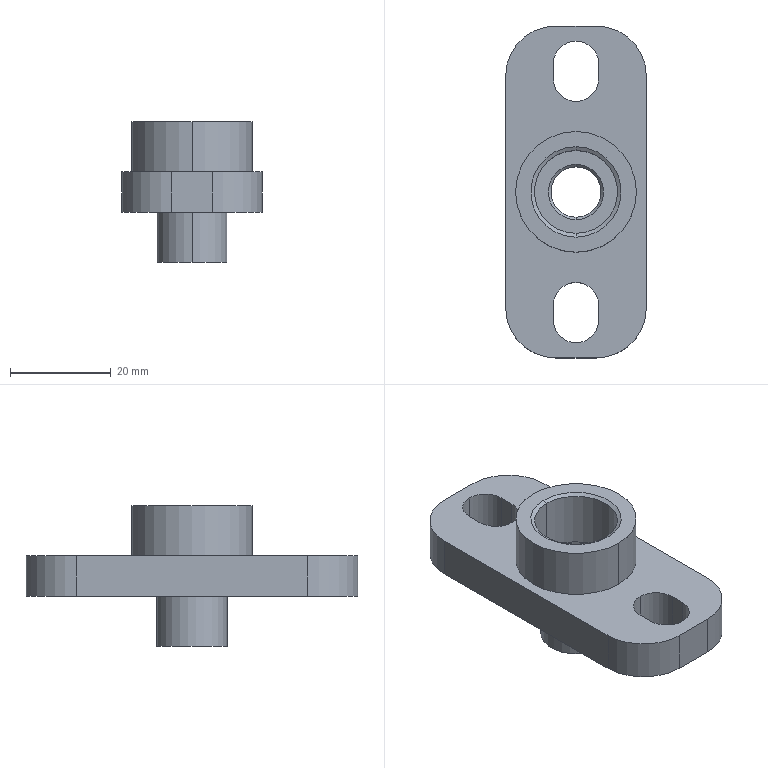Part | SolidWorks | features BaseBody 1 | 1 solid | 38 faces | box 28 x 66 x 28 mm | volume 14182 mm3 | cylinder 20 | plane 14 | cone 4 | commonest cylinder face diameters 9 x6 20 x4 10 x2 14 x2 16.5 x2 18.5 x2
STEP:
#1=CARTESIAN_POINT('',(172.5,-18.,46.8));
#2=VERTEX_POINT('',#1);
#3=CARTESIAN_POINT('',(168.,-22.5,46.8));
#4=VERTEX_POINT('',#3);
#5=CARTESIAN_POINT('',(172.5,-22.5,46.8));
#6=DIRECTION('',(0.,0.,1.));
#7=DIRECTION('',(0.,1.,0.));
#8=AXIS2_PLACEMENT_3D('',#5,#6,#7);
#9=CIRCLE('',#8,4.5);
#10=EDGE_CURVE('',#2,#4,#9,.T.);
#11=ORIENTED_EDGE('',*,*,#10,.F.);
#12=CARTESIAN_POINT('',(172.5,-18.,54.8));
#13=VERTEX_POINT('',#12);
#14=CARTESIAN_POINT('',(172.5,-18.,36.8));
#15=DIRECTION('',(0.,0.,1.));
#16=VECTOR('',#15,1000.);
#17=LINE('',#14,#16);
#18=EDGE_CURVE('',#2,#13,#17,.T.);
#19=ORIENTED_EDGE('',*,*,#18,.T.);
#20=CARTESIAN_POINT('',(168.,-22.5,54.8));
#21=VERTEX_POINT('',#20);
#22=CARTESIAN_POINT('',(172.5,-22.5,54.8));
#23=DIRECTION('',(0.,0.,1.));
#24=DIRECTION('',(0.,1.,0.));
#25=AXIS2_PLACEMENT_3D('',#22,#23,#24);
#26=CIRCLE('',#25,4.5);
#27=EDGE_CURVE('',#13,#21,#26,.T.);
#28=ORIENTED_EDGE('',*,*,#27,.T.);
#29=CARTESIAN_POINT('',(168.,-22.5,36.8));
#30=DIRECTION('',(0.,0.,1.));
#31=VECTOR('',#30,1000.);
#32=LINE('',#29,#31);
#33=EDGE_CURVE('',#4,#21,#32,.T.);
#34=ORIENTED_EDGE('',*,*,#33,.F.);
#35=EDGE_LOOP('',(#11,#19,#28,#34));
#36=FACE_OUTER_BOUND('',#35,.T.);
#37=CARTESIAN_POINT('',(172.5,-22.5,36.8));
#38=DIRECTION('',(0.,0.,1.));
#39=DIRECTION('',(0.,1.,0.));
#40=AXIS2_PLACEMENT_3D('',#37,#38,#39);
#41=CYLINDRICAL_SURFACE('',#40,4.5);
#42=ADVANCED_FACE('',(#36),#41,.F.);
#43=CARTESIAN_POINT('',(172.5,30.,46.8));
#44=VERTEX_POINT('',#43);
#45=CARTESIAN_POINT('',(168.,25.5,46.8));
#46=VERTEX_POINT('',#45);
#47=CARTESIAN_POINT('',(172.5,25.5,46.8));
#48=DIRECTION('',(0.,0.,1.));
#49=DIRECTION('',(0.,1.,0.));
#50=AXIS2_PLACEMENT_3D('',#47,#48,#49);
#51=CIRCLE('',#50,4.5);
#52=EDGE_CURVE('',#44,#46,#51,.T.);
#53=ORIENTED_EDGE('',*,*,#52,.F.);
#54=CARTESIAN_POINT('',(172.5,30.,54.8));
#55=VERTEX_POINT('',#54);
#56=CARTESIAN_POINT('',(172.5,30.,36.8));
#57=DIRECTION('',(0.,0.,1.));
#58=VECTOR('',#57,1000.);
#59=LINE('',#56,#58);
#60=EDGE_CURVE('',#44,#55,#59,.T.);
#61=ORIENTED_EDGE('',*,*,#60,.T.);
#62=CARTESIAN_POINT('',(168.,25.5,54.8));
#63=VERTEX_POINT('',#62);
#64=CARTESIAN_POINT('',(172.5,25.5,54.8));
#65=DIRECTION('',(0.,0.,1.));
#66=DIRECTION('',(0.,-1.,0.));
#67=AXIS2_PLACEMENT_3D('',#64,#65,#66);
#68=CIRCLE('',#67,4.5);
#69=EDGE_CURVE('',#55,#63,#68,.T.);
#70=ORIENTED_EDGE('',*,*,#69,.T.);
#71=CARTESIAN_POINT('',(168.,25.5,36.8));
#72=DIRECTION('',(0.,0.,1.));
#73=VECTOR('',#72,1000.);
#74=LINE('',#71,#73);
#75=EDGE_CURVE('',#46,#63,#74,.T.);
#76=ORIENTED_EDGE('',*,*,#75,.F.);
#77=EDGE_LOOP('',(#53,#61,#70,#76));
#78=FACE_OUTER_BOUND('',#77,.T.);
#79=CARTESIAN_POINT('',(172.5,25.5,36.8));
#80=DIRECTION('',(0.,0.,1.));
#81=DIRECTION('',(0.,1.,0.));
#82=AXIS2_PLACEMENT_3D('',#79,#80,#81);
#83=CYLINDRICAL_SURFACE('',#82,4.5);
#84=ADVANCED_FACE('',(#78),#83,.F.);
#85=CARTESIAN_POINT('',(172.5,-9.25,49.3));
#86=VERTEX_POINT('',#85);
#87=CARTESIAN_POINT('',(172.5,9.25,49.3));
#88=VERTEX_POINT('',#87);
#89=CARTESIAN_POINT('',(172.5,0.,49.3));
#90=DIRECTION('',(0.,0.,1.));
#91=DIRECTION('',(0.,1.,0.));
#92=AXIS2_PLACEMENT_3D('',#89,#90,#91);
#93=CIRCLE('',#92,9.25);
#94=EDGE_CURVE('',#86,#88,#93,.T.);
#95=ORIENTED_EDGE('',*,*,#94,.F.);
#96=CARTESIAN_POINT('',(172.5,-9.25,53.3));
#97=VERTEX_POINT('',#96);
#98=CARTESIAN_POINT('',(172.5,-9.25,65.548));
#99=DIRECTION('',(0.,0.,1.));
#100=VECTOR('',#99,1000.);
#101=LINE('',#98,#100);
#102=EDGE_CURVE('',#86,#97,#101,.T.);
#103=ORIENTED_EDGE('',*,*,#102,.T.);
#104=CARTESIAN_POINT('',(172.5,9.25,53.3));
#105=VERTEX_POINT('',#104);
#106=CARTESIAN_POINT('',(172.5,0.,53.3));
#107=DIRECTION('',(0.,0.,1.));
#108=DIRECTION('',(0.,1.,0.));
#109=AXIS2_PLACEMENT_3D('',#106,#107,#108);
#110=CIRCLE('',#109,9.25);
#111=EDGE_CURVE('',#97,#105,#110,.T.);
#112=ORIENTED_EDGE('',*,*,#111,.T.);
#113=CARTESIAN_POINT('',(172.5,9.25,65.548));
#114=DIRECTION('',(0.,0.,1.));
#115=VECTOR('',#114,1000.);
#116=LINE('',#113,#115);
#117=EDGE_CURVE('',#88,#105,#116,.T.);
#118=ORIENTED_EDGE('',*,*,#117,.F.);
#119=EDGE_LOOP('',(#95,#103,#112,#118));
#120=FACE_OUTER_BOUND('',#119,.T.);
#121=CARTESIAN_POINT('',(172.5,0.,65.548));
#122=DIRECTION('',(0.,0.,1.));
#123=DIRECTION('',(0.,1.,0.));
#124=AXIS2_PLACEMENT_3D('',#121,#122,#123);
#125=CYLINDRICAL_SURFACE('',#124,9.25);
#126=ADVANCED_FACE('',(#120),#125,.F.);
#127=CARTESIAN_POINT('',(172.5,-5.,48.8));
#128=VERTEX_POINT('',#127);
#129=CARTESIAN_POINT('',(172.5,5.,48.8));
#130=VERTEX_POINT('',#129);
#131=CARTESIAN_POINT('',(172.5,0.,48.8));
#132=DIRECTION('',(0.,0.,1.));
#133=DIRECTION('',(0.,-1.,0.));
#134=AXIS2_PLACEMENT_3D('',#131,#132,#133);
#135=CIRCLE('',#134,5.);
#136=EDGE_CURVE('',#128,#130,#135,.T.);
#137=ORIENTED_EDGE('',*,*,#136,.F.);
#138=CARTESIAN_POINT('',(172.5,-5.5,49.3));
#139=VERTEX_POINT('',#138);
#140=CARTESIAN_POINT('',(172.5,-5.,48.8));
#141=DIRECTION('',(0.,-0.7071,0.7071));
#142=VECTOR('',#141,1000.);
#143=LINE('',#140,#142);
#144=EDGE_CURVE('',#128,#139,#143,.T.);
#145=ORIENTED_EDGE('',*,*,#144,.T.);
#146=CARTESIAN_POINT('',(172.5,5.5,49.3));
#147=VERTEX_POINT('',#146);
#148=CARTESIAN_POINT('',(172.5,0.,49.3));
#149=DIRECTION('',(0.,0.,-1.));
#150=DIRECTION('',(0.,-1.,0.));
#151=AXIS2_PLACEMENT_3D('',#148,#149,#150);
#152=CIRCLE('',#151,5.5);
#153=EDGE_CURVE('',#147,#139,#152,.T.);
#154=ORIENTED_EDGE('',*,*,#153,.F.);
#155=CARTESIAN_POINT('',(172.5,5.,48.8));
#156=DIRECTION('',(0.,0.7071,0.7071));
#157=VECTOR('',#156,1000.);
#158=LINE('',#155,#157);
#159=EDGE_CURVE('',#130,#147,#158,.T.);
#160=ORIENTED_EDGE('',*,*,#159,.F.);
#161=EDGE_LOOP('',(#137,#145,#154,#160));
#162=FACE_OUTER_BOUND('',#161,.T.);
#163=CARTESIAN_POINT('',(172.5,0.,48.8));
#164=DIRECTION('',(0.,0.,1.));
#165=DIRECTION('',(0.,1.,0.));
#166=AXIS2_PLACEMENT_3D('',#163,#164,#165);
#167=CONICAL_SURFACE('',#166,5.,0.7854);
#168=ADVANCED_FACE('',(#162),#167,.F.);
#169=CARTESIAN_POINT('',(172.5,-8.25,64.367));
#170=VERTEX_POINT('',#169);
#171=CARTESIAN_POINT('',(172.5,8.25,64.367));
#172=VERTEX_POINT('',#171);
#173=CARTESIAN_POINT('',(172.5,0.,64.367));
#174=DIRECTION('',(0.,0.,1.));
#175=DIRECTION('',(0.,1.,0.));
#176=AXIS2_PLACEMENT_3D('',#173,#174,#175);
#177=CIRCLE('',#176,8.25);
#178=EDGE_CURVE('',#170,#172,#177,.T.);
#179=ORIENTED_EDGE('',*,*,#178,.F.);
#180=CARTESIAN_POINT('',(172.5,-9.,64.8));
#181=VERTEX_POINT('',#180);
#182=CARTESIAN_POINT('',(172.5,-9.,64.8));
#183=DIRECTION('',(0.,-0.866,0.5));
#184=VECTOR('',#183,1000.);
#185=LINE('',#182,#184);
#186=EDGE_CURVE('',#170,#181,#185,.T.);
#187=ORIENTED_EDGE('',*,*,#186,.T.);
#188=CARTESIAN_POINT('',(172.5,9.,64.8));
#189=VERTEX_POINT('',#188);
#190=CARTESIAN_POINT('',(172.5,0.,64.8));
#191=DIRECTION('',(0.,0.,1.));
#192=DIRECTION('',(0.,1.,0.));
#193=AXIS2_PLACEMENT_3D('',#190,#191,#192);
#194=CIRCLE('',#193,9.);
#195=EDGE_CURVE('',#181,#189,#194,.T.);
#196=ORIENTED_EDGE('',*,*,#195,.T.);
#197=CARTESIAN_POINT('',(172.5,9.,64.8));
#198=DIRECTION('',(0.,0.866,0.5));
#199=VECTOR('',#198,1000.);
#200=LINE('',#197,#199);
#201=EDGE_CURVE('',#172,#189,#200,.T.);
#202=ORIENTED_EDGE('',*,*,#201,.F.);
#203=EDGE_LOOP('',(#179,#187,#196,#202));
#204=FACE_OUTER_BOUND('',#203,.T.);
#205=CARTESIAN_POINT('',(172.5,0.,64.8));
#206=DIRECTION('',(0.,0.,1.));
#207=DIRECTION('',(0.,1.,0.));
#208=AXIS2_PLACEMENT_3D('',#205,#206,#207);
#209=CONICAL_SURFACE('',#208,9.,1.047);
#210=ADVANCED_FACE('',(#204),#209,.F.);
#211=CARTESIAN_POINT('',(172.5,-5.,36.8));
#212=VERTEX_POINT('',#211);
#213=CARTESIAN_POINT('',(172.5,5.,36.8));
#214=VERTEX_POINT('',#213);
#215=CARTESIAN_POINT('',(172.5,0.,36.8));
#216=DIRECTION('',(0.,0.,1.));
#217=DIRECTION('',(0.,1.,0.));
#218=AXIS2_PLACEMENT_3D('',#215,#216,#217);
#219=CIRCLE('',#218,5.);
#220=EDGE_CURVE('',#212,#214,#219,.T.);
#221=ORIENTED_EDGE('',*,*,#220,.F.);
#222=CARTESIAN_POINT('',(172.5,-5.,36.8));
#223=DIRECTION('',(0.,0.,1.));
#224=VECTOR('',#223,1000.);
#225=LINE('',#222,#224);
#226=EDGE_CURVE('',#212,#128,#225,.T.);
#227=ORIENTED_EDGE('',*,*,#226,.T.);
#228=ORIENTED_EDGE('',*,*,#136,.T.);
#229=CARTESIAN_POINT('',(172.5,5.,36.8));
#230=DIRECTION('',(0.,0.,1.));
#231=VECTOR('',#230,1000.);
#232=LINE('',#229,#231);
#233=EDGE_CURVE('',#214,#130,#232,.T.);
#234=ORIENTED_EDGE('',*,*,#233,.F.);
#235=EDGE_LOOP('',(#221,#227,#228,#234));
#236=FACE_OUTER_BOUND('',#235,.T.);
#237=CARTESIAN_POINT('',(172.5,0.,36.8));
#238=DIRECTION('',(0.,0.,1.));
#239=DIRECTION('',(0.,1.,0.));
#240=AXIS2_PLACEMENT_3D('',#237,#238,#239);
#241=CYLINDRICAL_SURFACE('',#240,5.);
#242=ADVANCED_FACE('',(#236),#241,.F.);
#243=CARTESIAN_POINT('',(172.5,7.,36.8));
#244=VERTEX_POINT('',#243);
#245=CARTESIAN_POINT('',(172.5,-7.,36.8));
#246=VERTEX_POINT('',#245);
#247=CARTESIAN_POINT('',(172.5,0.,36.8));
#248=DIRECTION('',(0.,0.,1.));
#249=DIRECTION('',(0.,1.,0.));
#250=AXIS2_PLACEMENT_3D('',#247,#248,#249);
#251=CIRCLE('',#250,7.);
#252=EDGE_CURVE('',#244,#246,#251,.T.);
#253=ORIENTED_EDGE('',*,*,#252,.T.);
#254=CARTESIAN_POINT('',(172.5,-7.,46.8));
#255=VERTEX_POINT('',#254);
#256=CARTESIAN_POINT('',(172.5,-7.,-10.999));
#257=DIRECTION('',(0.,0.,1.));
#258=VECTOR('',#257,1000.);
#259=LINE('',#256,#258);
#260=EDGE_CURVE('',#246,#255,#259,.T.);
#261=ORIENTED_EDGE('',*,*,#260,.T.);
#262=CARTESIAN_POINT('',(172.5,7.,46.8));
#263=VERTEX_POINT('',#262);
#264=CARTESIAN_POINT('',(172.5,0.,46.8));
#265=DIRECTION('',(0.,0.,-1.));
#266=DIRECTION('',(0.,1.,0.));
#267=AXIS2_PLACEMENT_3D('',#264,#265,#266);
#268=CIRCLE('',#267,7.);
#269=EDGE_CURVE('',#255,#263,#268,.T.);
#270=ORIENTED_EDGE('',*,*,#269,.T.);
#271=CARTESIAN_POINT('',(172.5,7.,-10.999));
#272=DIRECTION('',(0.,0.,1.));
#273=VECTOR('',#272,1000.);
#274=LINE('',#271,#273);
#275=EDGE_CURVE('',#244,#263,#274,.T.);
#276=ORIENTED_EDGE('',*,*,#275,.F.);
#277=EDGE_LOOP('',(#253,#261,#270,#276));
#278=FACE_OUTER_BOUND('',#277,.T.);
#279=CARTESIAN_POINT('',(172.5,0.,-10.999));
#280=DIRECTION('',(0.,0.,1.));
#281=DIRECTION('',(0.,1.,0.));
#282=AXIS2_PLACEMENT_3D('',#279,#280,#281);
#283=CYLINDRICAL_SURFACE('',#282,7.);
#284=ADVANCED_FACE('',(#278),#283,.T.);
#285=CARTESIAN_POINT('',(172.5,12.,64.8));
#286=VERTEX_POINT('',#285);
#287=CARTESIAN_POINT('',(172.5,-12.,64.8));
#288=VERTEX_POINT('',#287);
#289=CARTESIAN_POINT('',(172.5,0.,64.8));
#290=DIRECTION('',(0.,0.,1.));
#291=DIRECTION('',(0.,1.,0.));
#292=AXIS2_PLACEMENT_3D('',#289,#290,#291);
#293=CIRCLE('',#292,12.);
#294=EDGE_CURVE('',#286,#288,#293,.T.);
#295=ORIENTED_EDGE('',*,*,#294,.F.);
#296=CARTESIAN_POINT('',(172.5,12.,54.8));
#297=VERTEX_POINT('',#296);
#298=CARTESIAN_POINT('',(172.5,12.,64.8));
#299=DIRECTION('',(0.,0.,-1.));
#300=VECTOR('',#299,1000.);
#301=LINE('',#298,#300);
#302=EDGE_CURVE('',#286,#297,#301,.T.);
#303=ORIENTED_EDGE('',*,*,#302,.T.);
#304=CARTESIAN_POINT('',(172.5,-12.,54.8));
#305=VERTEX_POINT('',#304);
#306=CARTESIAN_POINT('',(172.5,0.,54.8));
#307=DIRECTION('',(0.,0.,1.));
#308=DIRECTION('',(0.,1.,0.));
#309=AXIS2_PLACEMENT_3D('',#306,#307,#308);
#310=CIRCLE('',#309,12.);
#311=EDGE_CURVE('',#297,#305,#310,.T.);
#312=ORIENTED_EDGE('',*,*,#311,.T.);
#313=CARTESIAN_POINT('',(172.5,-12.,64.8));
#314=DIRECTION('',(0.,0.,-1.));
#315=VECTOR('',#314,1000.);
#316=LINE('',#313,#315);
#317=EDGE_CURVE('',#288,#305,#316,.T.);
#318=ORIENTED_EDGE('',*,*,#317,.F.);
#319=EDGE_LOOP('',(#295,#303,#312,#318));
#320=FACE_OUTER_BOUND('',#319,.T.);
#321=CARTESIAN_POINT('',(172.5,0.,64.8));
#322=DIRECTION('',(0.,0.,-1.));
#323=DIRECTION('',(0.,-1.,0.));
#324=AXIS2_PLACEMENT_3D('',#321,#322,#323);
#325=CYLINDRICAL_SURFACE('',#324,12.);
#326=ADVANCED_FACE('',(#320),#325,.T.);
#327=CARTESIAN_POINT('',(172.5,-8.25,53.3));
#328=VERTEX_POINT('',#327);
#329=CARTESIAN_POINT('',(172.5,8.25,53.3));
#330=VERTEX_POINT('',#329);
#331=CARTESIAN_POINT('',(172.5,0.,53.3));
#332=DIRECTION('',(0.,0.,1.));
#333=DIRECTION('',(0.,-1.,0.));
#334=AXIS2_PLACEMENT_3D('',#331,#332,#333);
#335=CIRCLE('',#334,8.25);
#336=EDGE_CURVE('',#328,#330,#335,.T.);
#337=ORIENTED_EDGE('',*,*,#336,.F.);
#338=CARTESIAN_POINT('',(172.5,-8.25,64.8));
#339=DIRECTION('',(0.,0.,1.));
#340=VECTOR('',#339,1000.);
#341=LINE('',#338,#340);
#342=EDGE_CURVE('',#328,#170,#341,.T.);
#343=ORIENTED_EDGE('',*,*,#342,.T.);
#344=ORIENTED_EDGE('',*,*,#178,.T.);
#345=CARTESIAN_POINT('',(172.5,8.25,64.8));
#346=DIRECTION('',(0.,0.,1.));
#347=VECTOR('',#346,1000.);
#348=LINE('',#345,#347);
#349=EDGE_CURVE('',#330,#172,#348,.T.);
#350=ORIENTED_EDGE('',*,*,#349,.F.);
#351=EDGE_LOOP('',(#337,#343,#344,#350));
#352=FACE_OUTER_BOUND('',#351,.T.);
#353=CARTESIAN_POINT('',(172.5,0.,64.8));
#354=DIRECTION('',(0.,0.,1.));
#355=DIRECTION('',(0.,1.,0.));
#356=AXIS2_PLACEMENT_3D('',#353,#354,#355);
#357=CYLINDRICAL_SURFACE('',#356,8.25);
#358=ADVANCED_FACE('',(#352),#357,.F.);
#359=ORIENTED_EDGE('',*,*,#342,.F.);
#360=CARTESIAN_POINT('',(172.5,0.,53.3));
#361=DIRECTION('',(0.,0.,1.));
#362=DIRECTION('',(0.,-1.,0.));
#363=AXIS2_PLACEMENT_3D('',#360,#361,#362);
#364=CIRCLE('',#363,8.25);
#365=EDGE_CURVE('',#330,#328,#364,.T.);
#366=ORIENTED_EDGE('',*,*,#365,.F.);
#367=ORIENTED_EDGE('',*,*,#349,.T.);
#368=CARTESIAN_POINT('',(172.5,0.,64.367));
#369=DIRECTION('',(0.,0.,1.));
#370=DIRECTION('',(0.,1.,0.));
#371=AXIS2_PLACEMENT_3D('',#368,#369,#370);
#372=CIRCLE('',#371,8.25);
#373=EDGE_CURVE('',#172,#170,#372,.T.);
#374=ORIENTED_EDGE('',*,*,#373,.T.);
#375=EDGE_LOOP('',(#359,#366,#367,#374));
#376=FACE_OUTER_BOUND('',#375,.T.);
#377=CARTESIAN_POINT('',(172.5,0.,64.8));
#378=DIRECTION('',(0.,0.,1.));
#379=DIRECTION('',(0.,1.,0.));
#380=AXIS2_PLACEMENT_3D('',#377,#378,#379);
#381=CYLINDRICAL_SURFACE('',#380,8.25);
#382=ADVANCED_FACE('',(#376),#381,.F.);
#383=CARTESIAN_POINT('',(168.,-25.5,46.8));
#384=VERTEX_POINT('',#383);
#385=CARTESIAN_POINT('',(168.,23.,46.8));
#386=DIRECTION('',(0.,-1.,0.));
#387=VECTOR('',#386,1000.);
#388=LINE('',#385,#387);
#389=EDGE_CURVE('',#4,#384,#388,.T.);
#390=ORIENTED_EDGE('',*,*,#389,.T.);
#391=CARTESIAN_POINT('',(177.,-25.5,46.8));
#392=VERTEX_POINT('',#391);
#393=CARTESIAN_POINT('',(172.5,-25.5,46.8));
#394=DIRECTION('',(0.,0.,1.));
#395=DIRECTION('',(0.,1.,0.));
#396=AXIS2_PLACEMENT_3D('',#393,#394,#395);
#397=CIRCLE('',#396,4.5);
#398=EDGE_CURVE('',#384,#392,#397,.T.);
#399=ORIENTED_EDGE('',*,*,#398,.T.);
#400=CARTESIAN_POINT('',(177.,-22.5,46.8));
#401=VERTEX_POINT('',#400);
#402=CARTESIAN_POINT('',(177.,23.,46.8));
#403=DIRECTION('',(0.,1.,0.));
#404=VECTOR('',#403,1000.);
#405=LINE('',#402,#404);
#406=EDGE_CURVE('',#392,#401,#405,.T.);
#407=ORIENTED_EDGE('',*,*,#406,.T.);
#408=CARTESIAN_POINT('',(172.5,-22.5,46.8));
#409=DIRECTION('',(0.,0.,1.));
#410=DIRECTION('',(0.,1.,0.));
#411=AXIS2_PLACEMENT_3D('',#408,#409,#410);
#412=CIRCLE('',#411,4.5);
#413=EDGE_CURVE('',#401,#2,#412,.T.);
#414=ORIENTED_EDGE('',*,*,#413,.T.);
#415=ORIENTED_EDGE('',*,*,#10,.T.);
#416=EDGE_LOOP('',(#390,#399,#407,#414,#415));
#417=FACE_BOUND('',#416,.T.);
#418=CARTESIAN_POINT('',(168.,22.5,46.8));
#419=VERTEX_POINT('',#418);
#420=CARTESIAN_POINT('',(168.,23.,46.8));
#421=DIRECTION('',(0.,-1.,0.));
#422=VECTOR('',#421,1000.);
#423=LINE('',#420,#422);
#424=EDGE_CURVE('',#46,#419,#423,.T.);
#425=ORIENTED_EDGE('',*,*,#424,.T.);
#426=CARTESIAN_POINT('',(177.,22.5,46.8));
#427=VERTEX_POINT('',#426);
#428=CARTESIAN_POINT('',(172.5,22.5,46.8));
#429=DIRECTION('',(0.,0.,1.));
#430=DIRECTION('',(0.,1.,0.));
#431=AXIS2_PLACEMENT_3D('',#428,#429,#430);
#432=CIRCLE('',#431,4.5);
#433=EDGE_CURVE('',#419,#427,#432,.T.);
#434=ORIENTED_EDGE('',*,*,#433,.T.);
#435=CARTESIAN_POINT('',(177.,25.5,46.8));
#436=VERTEX_POINT('',#435);
#437=CARTESIAN_POINT('',(177.,23.,46.8));
#438=DIRECTION('',(0.,1.,0.));
#439=VECTOR('',#438,1000.);
#440=LINE('',#437,#439);
#441=EDGE_CURVE('',#427,#436,#440,.T.);
#442=ORIENTED_EDGE('',*,*,#441,.T.);
#443=CARTESIAN_POINT('',(172.5,25.5,46.8));
#444=DIRECTION('',(0.,0.,1.));
#445=DIRECTION('',(0.,1.,0.));
#446=AXIS2_PLACEMENT_3D('',#443,#444,#445);
#447=CIRCLE('',#446,4.5);
#448=EDGE_CURVE('',#436,#44,#447,.T.);
#449=ORIENTED_EDGE('',*,*,#448,.T.);
#450=ORIENTED_EDGE('',*,*,#52,.T.);
#451=EDGE_LOOP('',(#425,#434,#442,#449,#450));
#452=FACE_BOUND('',#451,.T.);
#453=CARTESIAN_POINT('',(168.5,33.,46.8));
#454=VERTEX_POINT('',#453);
#455=CARTESIAN_POINT('',(158.5,23.,46.8));
#456=VERTEX_POINT('',#455);
#457=CARTESIAN_POINT('',(168.5,23.,46.8));
#458=DIRECTION('',(0.,0.,1.));
#459=DIRECTION('',(0.,1.,0.));
#460=AXIS2_PLACEMENT_3D('',#457,#458,#459);
#461=CIRCLE('',#460,10.);
#462=EDGE_CURVE('',#454,#456,#461,.T.);
#463=ORIENTED_EDGE('',*,*,#462,.F.);
#464=CARTESIAN_POINT('',(176.5,33.,46.8));
#465=VERTEX_POINT('',#464);
#466=CARTESIAN_POINT('',(168.5,33.,46.8));
#467=DIRECTION('',(-1.,0.,0.));
#468=VECTOR('',#467,1000.);
#469=LINE('',#466,#468);
#470=EDGE_CURVE('',#465,#454,#469,.T.);
#471=ORIENTED_EDGE('',*,*,#470,.F.);
#472=CARTESIAN_POINT('',(186.5,23.,46.8));
#473=VERTEX_POINT('',#472);
#474=CARTESIAN_POINT('',(176.5,23.,46.8));
#475=DIRECTION('',(0.,0.,1.));
#476=DIRECTION('',(0.,1.,0.));
#477=AXIS2_PLACEMENT_3D('',#474,#475,#476);
#478=CIRCLE('',#477,10.);
#479=EDGE_CURVE('',#473,#465,#478,.T.);
#480=ORIENTED_EDGE('',*,*,#479,.F.);
#481=CARTESIAN_POINT('',(186.5,-23.,46.8));
#482=VERTEX_POINT('',#481);
#483=CARTESIAN_POINT('',(186.5,-23.,46.8));
#484=DIRECTION('',(0.,1.,0.));
#485=VECTOR('',#484,1000.);
#486=LINE('',#483,#485);
#487=EDGE_CURVE('',#482,#473,#486,.T.);
#488=ORIENTED_EDGE('',*,*,#487,.F.);
#489=CARTESIAN_POINT('',(176.5,-33.,46.8));
#490=VERTEX_POINT('',#489);
#491=CARTESIAN_POINT('',(176.5,-23.,46.8));
#492=DIRECTION('',(0.,0.,1.));
#493=DIRECTION('',(0.,1.,0.));
#494=AXIS2_PLACEMENT_3D('',#491,#492,#493);
#495=CIRCLE('',#494,10.);
#496=EDGE_CURVE('',#490,#482,#495,.T.);
#497=ORIENTED_EDGE('',*,*,#496,.F.);
#498=CARTESIAN_POINT('',(168.5,-33.,46.8));
#499=VERTEX_POINT('',#498);
#500=CARTESIAN_POINT('',(168.5,-33.,46.8));
#501=DIRECTION('',(1.,0.,0.));
#502=VECTOR('',#501,1000.);
#503=LINE('',#500,#502);
#504=EDGE_CURVE('',#499,#490,#503,.T.);
#505=ORIENTED_EDGE('',*,*,#504,.F.);
#506=CARTESIAN_POINT('',(158.5,-23.,46.8));
#507=VERTEX_POINT('',#506);
#508=CARTESIAN_POINT('',(168.5,-23.,46.8));
#509=DIRECTION('',(0.,0.,1.));
#510=DIRECTION('',(0.,1.,0.));
#511=AXIS2_PLACEMENT_3D('',#508,#509,#510);
#512=CIRCLE('',#511,10.);
#513=EDGE_CURVE('',#507,#499,#512,.T.);
#514=ORIENTED_EDGE('',*,*,#513,.F.);
#515=CARTESIAN_POINT('',(158.5,-23.,46.8));
#516=DIRECTION('',(0.,-1.,0.));
#517=VECTOR('',#516,1000.);
#518=LINE('',#515,#517);
#519=EDGE_CURVE('',#456,#507,#518,.T.);
#520=ORIENTED_EDGE('',*,*,#519,.F.);
#521=EDGE_LOOP('',(#463,#471,#480,#488,#497,#505,#514,#520));
#522=FACE_OUTER_BOUND('',#521,.T.);
#523=CARTESIAN_POINT('',(172.5,0.,46.8));
#524=DIRECTION('',(0.,0.,-1.));
#525=DIRECTION('',(0.,1.,0.));
#526=AXIS2_PLACEMENT_3D('',#523,#524,#525);
#527=CIRCLE('',#526,7.);
#528=EDGE_CURVE('',#263,#255,#527,.T.);
#529=ORIENTED_EDGE('',*,*,#528,.F.);
#530=ORIENTED_EDGE('',*,*,#269,.F.);
#531=EDGE_LOOP('',(#529,#530));
#532=FACE_BOUND('',#531,.T.);
#533=CARTESIAN_POINT('',(168.5,23.,46.8));
#534=DIRECTION('',(0.,0.,1.));
#535=DIRECTION('',(0.,1.,0.));
#536=AXIS2_PLACEMENT_3D('',#533,#534,#535);
#537=PLANE('',#536);
#538=ADVANCED_FACE('',(#417,#452,#522,#532),#537,.F.);
#539=CARTESIAN_POINT('',(168.,-25.5,54.8));
#540=VERTEX_POINT('',#539);
#541=CARTESIAN_POINT('',(177.,-25.5,54.8));
#542=VERTEX_POINT('',#541);
#543=CARTESIAN_POINT('',(172.5,-25.5,54.8));
#544=DIRECTION('',(0.,0.,1.));
#545=DIRECTION('',(0.,1.,0.));
#546=AXIS2_PLACEMENT_3D('',#543,#544,#545);
#547=CIRCLE('',#546,4.5);
#548=EDGE_CURVE('',#540,#542,#547,.T.);
#549=ORIENTED_EDGE('',*,*,#548,.F.);
#550=CARTESIAN_POINT('',(168.,-25.5,54.8));
#551=DIRECTION('',(0.,-1.,0.));
#552=VECTOR('',#551,1000.);
#553=LINE('',#550,#552);
#554=EDGE_CURVE('',#21,#540,#553,.T.);
#555=ORIENTED_EDGE('',*,*,#554,.F.);
#556=ORIENTED_EDGE('',*,*,#27,.F.);
#557=CARTESIAN_POINT('',(177.,-22.5,54.8));
#558=VERTEX_POINT('',#557);
#559=CARTESIAN_POINT('',(172.5,-22.5,54.8));
#560=DIRECTION('',(0.,0.,1.));
#561=DIRECTION('',(0.,1.,0.));
#562=AXIS2_PLACEMENT_3D('',#559,#560,#561);
#563=CIRCLE('',#562,4.5);
#564=EDGE_CURVE('',#558,#13,#563,.T.);
#565=ORIENTED_EDGE('',*,*,#564,.F.);
#566=CARTESIAN_POINT('',(177.,-22.5,54.8));
#567=DIRECTION('',(0.,1.,0.));
#568=VECTOR('',#567,1000.);
#569=LINE('',#566,#568);
#570=EDGE_CURVE('',#542,#558,#569,.T.);
#571=ORIENTED_EDGE('',*,*,#570,.F.);
#572=EDGE_LOOP('',(#549,#555,#556,#565,#571));
#573=FACE_BOUND('',#572,.T.);
#574=CARTESIAN_POINT('',(168.,22.5,54.8));
#575=VERTEX_POINT('',#574);
#576=CARTESIAN_POINT('',(177.,22.5,54.8));
#577=VERTEX_POINT('',#576);
#578=CARTESIAN_POINT('',(172.5,22.5,54.8));
#579=DIRECTION('',(0.,0.,1.));
#580=DIRECTION('',(0.,-1.,0.));
#581=AXIS2_PLACEMENT_3D('',#578,#579,#580);
#582=CIRCLE('',#581,4.5);
#583=EDGE_CURVE('',#575,#577,#582,.T.);
#584=ORIENTED_EDGE('',*,*,#583,.F.);
#585=CARTESIAN_POINT('',(168.,25.5,54.8));
#586=DIRECTION('',(0.,-1.,0.));
#587=VECTOR('',#586,1000.);
#588=LINE('',#585,#587);
#589=EDGE_CURVE('',#63,#575,#588,.T.);
#590=ORIENTED_EDGE('',*,*,#589,.F.);
#591=ORIENTED_EDGE('',*,*,#69,.F.);
#592=CARTESIAN_POINT('',(177.,25.5,54.8));
#593=VERTEX_POINT('',#592);
#594=CARTESIAN_POINT('',(172.5,25.5,54.8));
#595=DIRECTION('',(0.,0.,1.));
#596=DIRECTION('',(0.,-1.,0.));
#597=AXIS2_PLACEMENT_3D('',#594,#595,#596);
#598=CIRCLE('',#597,4.5);
#599=EDGE_CURVE('',#593,#55,#598,.T.);
#600=ORIENTED_EDGE('',*,*,#599,.F.);
#601=CARTESIAN_POINT('',(177.,22.5,54.8));
#602=DIRECTION('',(0.,1.,0.));
#603=VECTOR('',#602,1000.);
#604=LINE('',#601,#603);
#605=EDGE_CURVE('',#577,#593,#604,.T.);
#606=ORIENTED_EDGE('',*,*,#605,.F.);
#607=EDGE_LOOP('',(#584,#590,#591,#600,#606));
#608=FACE_BOUND('',#607,.T.);
#609=CARTESIAN_POINT('',(168.5,33.,54.8));
#610=VERTEX_POINT('',#609);
#611=CARTESIAN_POINT('',(158.5,23.,54.8));
#612=VERTEX_POINT('',#611);
#613=CARTESIAN_POINT('',(168.5,23.,54.8));
#614=DIRECTION('',(0.,0.,1.));
#615=DIRECTION('',(0.,1.,0.));
#616=AXIS2_PLACEMENT_3D('',#613,#614,#615);
#617=CIRCLE('',#616,10.);
#618=EDGE_CURVE('',#610,#612,#617,.T.);
#619=ORIENTED_EDGE('',*,*,#618,.T.);
#620=CARTESIAN_POINT('',(158.5,-23.,54.8));
#621=VERTEX_POINT('',#620);
#622=CARTESIAN_POINT('',(158.5,-23.,54.8));
#623=DIRECTION('',(0.,-1.,0.));
#624=VECTOR('',#623,1000.);
#625=LINE('',#622,#624);
#626=EDGE_CURVE('',#612,#621,#625,.T.);
#627=ORIENTED_EDGE('',*,*,#626,.T.);
#628=CARTESIAN_POINT('',(168.5,-33.,54.8));
#629=VERTEX_POINT('',#628);
#630=CARTESIAN_POINT('',(168.5,-23.,54.8));
#631=DIRECTION('',(0.,0.,1.));
#632=DIRECTION('',(0.,1.,0.));
#633=AXIS2_PLACEMENT_3D('',#630,#631,#632);
#634=CIRCLE('',#633,10.);
#635=EDGE_CURVE('',#621,#629,#634,.T.);
#636=ORIENTED_EDGE('',*,*,#635,.T.);
#637=CARTESIAN_POINT('',(176.5,-33.,54.8));
#638=VERTEX_POINT('',#637);
#639=CARTESIAN_POINT('',(168.5,-33.,54.8));
#640=DIRECTION('',(1.,0.,0.));
#641=VECTOR('',#640,1000.);
#642=LINE('',#639,#641);
#643=EDGE_CURVE('',#629,#638,#642,.T.);
#644=ORIENTED_EDGE('',*,*,#643,.T.);
#645=CARTESIAN_POINT('',(186.5,-23.,54.8));
#646=VERTEX_POINT('',#645);
#647=CARTESIAN_POINT('',(176.5,-23.,54.8));
#648=DIRECTION('',(0.,0.,1.));
#649=DIRECTION('',(0.,1.,0.));
#650=AXIS2_PLACEMENT_3D('',#647,#648,#649);
#651=CIRCLE('',#650,10.);
#652=EDGE_CURVE('',#638,#646,#651,.T.);
#653=ORIENTED_EDGE('',*,*,#652,.T.);
#654=CARTESIAN_POINT('',(186.5,23.,54.8));
#655=VERTEX_POINT('',#654);
#656=CARTESIAN_POINT('',(186.5,-23.,54.8));
#657=DIRECTION('',(0.,1.,0.));
#658=VECTOR('',#657,1000.);
#659=LINE('',#656,#658);
#660=EDGE_CURVE('',#646,#655,#659,.T.);
#661=ORIENTED_EDGE('',*,*,#660,.T.);
#662=CARTESIAN_POINT('',(176.5,33.,54.8));
#663=VERTEX_POINT('',#662);
#664=CARTESIAN_POINT('',(176.5,23.,54.8));
#665=DIRECTION('',(0.,0.,1.));
#666=DIRECTION('',(0.,1.,0.));
#667=AXIS2_PLACEMENT_3D('',#664,#665,#666);
#668=CIRCLE('',#667,10.);
#669=EDGE_CURVE('',#655,#663,#668,.T.);
#670=ORIENTED_EDGE('',*,*,#669,.T.);
#671=CARTESIAN_POINT('',(168.5,33.,54.8));
#672=DIRECTION('',(-1.,0.,0.));
#673=VECTOR('',#672,1000.);
#674=LINE('',#671,#673);
#675=EDGE_CURVE('',#663,#610,#674,.T.);
#676=ORIENTED_EDGE('',*,*,#675,.T.);
#677=EDGE_LOOP('',(#619,#627,#636,#644,#653,#661,#670,#676));
#678=FACE_OUTER_BOUND('',#677,.T.);
#679=CARTESIAN_POINT('',(172.5,0.,54.8));
#680=DIRECTION('',(0.,0.,1.));
#681=DIRECTION('',(0.,1.,0.));
#682=AXIS2_PLACEMENT_3D('',#679,#680,#681);
#683=CIRCLE('',#682,12.);
#684=EDGE_CURVE('',#305,#297,#683,.T.);
#685=ORIENTED_EDGE('',*,*,#684,.F.);
#686=ORIENTED_EDGE('',*,*,#311,.F.);
#687=EDGE_LOOP('',(#685,#686));
#688=FACE_BOUND('',#687,.T.);
#689=CARTESIAN_POINT('',(168.5,23.,54.8));
#690=DIRECTION('',(0.,0.,1.));
#691=DIRECTION('',(0.,1.,0.));
#692=AXIS2_PLACEMENT_3D('',#689,#690,#691);
#693=PLANE('',#692);
#694=ADVANCED_FACE('',(#573,#608,#678,#688),#693,.T.);
#695=ORIENTED_EDGE('',*,*,#462,.T.);
#696=CARTESIAN_POINT('',(158.5,23.,54.8));
#697=DIRECTION('',(0.,0.,-1.));
#698=VECTOR('',#697,1000.);
#699=LINE('',#696,#698);
#700=EDGE_CURVE('',#612,#456,#699,.T.);
#701=ORIENTED_EDGE('',*,*,#700,.F.);
#702=ORIENTED_EDGE('',*,*,#618,.F.);
#703=CARTESIAN_POINT('',(168.5,33.,54.8));
#704=DIRECTION('',(0.,0.,-1.));
#705=VECTOR('',#704,1000.);
#706=LINE('',#703,#705);
#707=EDGE_CURVE('',#610,#454,#706,.T.);
#708=ORIENTED_EDGE('',*,*,#707,.T.);
#709=EDGE_LOOP('',(#695,#701,#702,#708));
#710=FACE_OUTER_BOUND('',#709,.T.);
#711=CARTESIAN_POINT('',(168.5,23.,54.8));
#712=DIRECTION('',(0.,0.,-1.));
#713=DIRECTION('',(0.,-1.,0.));
#714=AXIS2_PLACEMENT_3D('',#711,#712,#713);
#715=CYLINDRICAL_SURFACE('',#714,10.);
#716=ADVANCED_FACE('',(#710),#715,.T.);
#717=ORIENTED_EDGE('',*,*,#519,.T.);
#718=CARTESIAN_POINT('',(158.5,-23.,54.8));
#719=DIRECTION('',(0.,0.,-1.));
#720=VECTOR('',#719,1000.);
#721=LINE('',#718,#720);
#722=EDGE_CURVE('',#621,#507,#721,.T.);
#723=ORIENTED_EDGE('',*,*,#722,.F.);
#724=ORIENTED_EDGE('',*,*,#626,.F.);
#725=ORIENTED_EDGE('',*,*,#700,.T.);
#726=EDGE_LOOP('',(#717,#723,#724,#725));
#727=FACE_OUTER_BOUND('',#726,.T.);
#728=CARTESIAN_POINT('',(158.5,-23.,54.8));
#729=DIRECTION('',(1.,0.,0.));
#730=DIRECTION('',(0.,1.,0.));
#731=AXIS2_PLACEMENT_3D('',#728,#729,#730);
#732=PLANE('',#731);
#733=ADVANCED_FACE('',(#727),#732,.F.);
#734=ORIENTED_EDGE('',*,*,#513,.T.);
#735=CARTESIAN_POINT('',(168.5,-33.,54.8));
#736=DIRECTION('',(0.,0.,-1.));
#737=VECTOR('',#736,1000.);
#738=LINE('',#735,#737);
#739=EDGE_CURVE('',#629,#499,#738,.T.);
#740=ORIENTED_EDGE('',*,*,#739,.F.);
#741=ORIENTED_EDGE('',*,*,#635,.F.);
#742=ORIENTED_EDGE('',*,*,#722,.T.);
#743=EDGE_LOOP('',(#734,#740,#741,#742));
#744=FACE_OUTER_BOUND('',#743,.T.);
#745=CARTESIAN_POINT('',(168.5,-23.,54.8));
#746=DIRECTION('',(0.,0.,-1.));
#747=DIRECTION('',(0.,-1.,0.));
#748=AXIS2_PLACEMENT_3D('',#745,#746,#747);
#749=CYLINDRICAL_SURFACE('',#748,10.);
#750=ADVANCED_FACE('',(#744),#749,.T.);
#751=ORIENTED_EDGE('',*,*,#504,.T.);
#752=CARTESIAN_POINT('',(176.5,-33.,54.8));
#753=DIRECTION('',(0.,0.,-1.));
#754=VECTOR('',#753,1000.);
#755=LINE('',#752,#754);
#756=EDGE_CURVE('',#638,#490,#755,.T.);
#757=ORIENTED_EDGE('',*,*,#756,.F.);
#758=ORIENTED_EDGE('',*,*,#643,.F.);
#759=ORIENTED_EDGE('',*,*,#739,.T.);
#760=EDGE_LOOP('',(#751,#757,#758,#759));
#761=FACE_OUTER_BOUND('',#760,.T.);
#762=CARTESIAN_POINT('',(168.5,-33.,54.8));
#763=DIRECTION('',(0.,1.,0.));
#764=DIRECTION('',(0.,0.,-1.));
#765=AXIS2_PLACEMENT_3D('',#762,#763,#764);
#766=PLANE('',#765);
#767=ADVANCED_FACE('',(#761),#766,.F.);
#768=ORIENTED_EDGE('',*,*,#496,.T.);
#769=CARTESIAN_POINT('',(186.5,-23.,54.8));
#770=DIRECTION('',(0.,0.,-1.));
#771=VECTOR('',#770,1000.);
#772=LINE('',#769,#771);
#773=EDGE_CURVE('',#646,#482,#772,.T.);
#774=ORIENTED_EDGE('',*,*,#773,.F.);
#775=ORIENTED_EDGE('',*,*,#652,.F.);
#776=ORIENTED_EDGE('',*,*,#756,.T.);
#777=EDGE_LOOP('',(#768,#774,#775,#776));
#778=FACE_OUTER_BOUND('',#777,.T.);
#779=CARTESIAN_POINT('',(176.5,-23.,54.8));
#780=DIRECTION('',(0.,0.,-1.));
#781=DIRECTION('',(0.,-1.,0.));
#782=AXIS2_PLACEMENT_3D('',#779,#780,#781);
#783=CYLINDRICAL_SURFACE('',#782,10.);
#784=ADVANCED_FACE('',(#778),#783,.T.);
#785=ORIENTED_EDGE('',*,*,#487,.T.);
#786=CARTESIAN_POINT('',(186.5,23.,54.8));
#787=DIRECTION('',(0.,0.,-1.));
#788=VECTOR('',#787,1000.);
#789=LINE('',#786,#788);
#790=EDGE_CURVE('',#655,#473,#789,.T.);
#791=ORIENTED_EDGE('',*,*,#790,.F.);
#792=ORIENTED_EDGE('',*,*,#660,.F.);
#793=ORIENTED_EDGE('',*,*,#773,.T.);
#794=EDGE_LOOP('',(#785,#791,#792,#793));
#795=FACE_OUTER_BOUND('',#794,.T.);
#796=CARTESIAN_POINT('',(186.5,-23.,54.8));
#797=DIRECTION('',(-1.,0.,0.));
#798=DIRECTION('',(0.,-1.,0.));
#799=AXIS2_PLACEMENT_3D('',#796,#797,#798);
#800=PLANE('',#799);
#801=ADVANCED_FACE('',(#795),#800,.F.);
#802=ORIENTED_EDGE('',*,*,#479,.T.);
#803=CARTESIAN_POINT('',(176.5,33.,54.8));
#804=DIRECTION('',(0.,0.,-1.));
#805=VECTOR('',#804,1000.);
#806=LINE('',#803,#805);
#807=EDGE_CURVE('',#663,#465,#806,.T.);
#808=ORIENTED_EDGE('',*,*,#807,.F.);
#809=ORIENTED_EDGE('',*,*,#669,.F.);
#810=ORIENTED_EDGE('',*,*,#790,.T.);
#811=EDGE_LOOP('',(#802,#808,#809,#810));
#812=FACE_OUTER_BOUND('',#811,.T.);
#813=CARTESIAN_POINT('',(176.5,23.,54.8));
#814=DIRECTION('',(0.,0.,-1.));
#815=DIRECTION('',(0.,-1.,0.));
#816=AXIS2_PLACEMENT_3D('',#813,#814,#815);
#817=CYLINDRICAL_SURFACE('',#816,10.);
#818=ADVANCED_FACE('',(#812),#817,.T.);
#819=ORIENTED_EDGE('',*,*,#470,.T.);
#820=ORIENTED_EDGE('',*,*,#707,.F.);
#821=ORIENTED_EDGE('',*,*,#675,.F.);
#822=ORIENTED_EDGE('',*,*,#807,.T.);
#823=EDGE_LOOP('',(#819,#820,#821,#822));
#824=FACE_OUTER_BOUND('',#823,.T.);
#825=CARTESIAN_POINT('',(168.5,33.,54.8));
#826=DIRECTION('',(0.,-1.,0.));
#827=DIRECTION('',(0.,0.,1.));
#828=AXIS2_PLACEMENT_3D('',#825,#826,#827);
#829=PLANE('',#828);
#830=ADVANCED_FACE('',(#824),#829,.F.);
#831=ORIENTED_EDGE('',*,*,#302,.F.);
#832=CARTESIAN_POINT('',(172.5,0.,64.8));
#833=DIRECTION('',(0.,0.,1.));
#834=DIRECTION('',(0.,1.,0.));
#835=AXIS2_PLACEMENT_3D('',#832,#833,#834);
#836=CIRCLE('',#835,12.);
#837=EDGE_CURVE('',#288,#286,#836,.T.);
#838=ORIENTED_EDGE('',*,*,#837,.F.);
#839=ORIENTED_EDGE('',*,*,#317,.T.);
#840=ORIENTED_EDGE('',*,*,#684,.T.);
#841=EDGE_LOOP('',(#831,#838,#839,#840));
#842=FACE_OUTER_BOUND('',#841,.T.);
#843=CARTESIAN_POINT('',(172.5,0.,64.8));
#844=DIRECTION('',(0.,0.,-1.));
#845=DIRECTION('',(0.,-1.,0.));
#846=AXIS2_PLACEMENT_3D('',#843,#844,#845);
#847=CYLINDRICAL_SURFACE('',#846,12.);
#848=ADVANCED_FACE('',(#842),#847,.T.);
#849=CARTESIAN_POINT('',(172.5,0.,64.8));
#850=DIRECTION('',(0.,0.,1.));
#851=DIRECTION('',(0.,1.,0.));
#852=AXIS2_PLACEMENT_3D('',#849,#850,#851);
#853=CIRCLE('',#852,9.);
#854=EDGE_CURVE('',#189,#181,#853,.T.);
#855=ORIENTED_EDGE('',*,*,#854,.F.);
#856=ORIENTED_EDGE('',*,*,#195,.F.);
#857=EDGE_LOOP('',(#855,#856));
#858=FACE_BOUND('',#857,.T.);
#859=ORIENTED_EDGE('',*,*,#837,.T.);
#860=ORIENTED_EDGE('',*,*,#294,.T.);
#861=EDGE_LOOP('',(#859,#860));
#862=FACE_OUTER_BOUND('',#861,.T.);
#863=CARTESIAN_POINT('',(172.5,0.,64.8));
#864=DIRECTION('',(0.,0.,1.));
#865=DIRECTION('',(0.,1.,0.));
#866=AXIS2_PLACEMENT_3D('',#863,#864,#865);
#867=PLANE('',#866);
#868=ADVANCED_FACE('',(#858,#862),#867,.T.);
#869=ORIENTED_EDGE('',*,*,#260,.F.);
#870=CARTESIAN_POINT('',(172.5,0.,36.8));
#871=DIRECTION('',(0.,0.,1.));
#872=DIRECTION('',(0.,1.,0.));
#873=AXIS2_PLACEMENT_3D('',#870,#871,#872);
#874=CIRCLE('',#873,7.);
#875=EDGE_CURVE('',#246,#244,#874,.T.);
#876=ORIENTED_EDGE('',*,*,#875,.T.);
#877=ORIENTED_EDGE('',*,*,#275,.T.);
#878=ORIENTED_EDGE('',*,*,#528,.T.);
#879=EDGE_LOOP('',(#869,#876,#877,#878));
#880=FACE_OUTER_BOUND('',#879,.T.);
#881=CARTESIAN_POINT('',(172.5,0.,-10.999));
#882=DIRECTION('',(0.,0.,1.));
#883=DIRECTION('',(0.,1.,0.));
#884=AXIS2_PLACEMENT_3D('',#881,#882,#883);
#885=CYLINDRICAL_SURFACE('',#884,7.);
#886=ADVANCED_FACE('',(#880),#885,.T.);
#887=CARTESIAN_POINT('',(172.5,0.,36.8));
#888=DIRECTION('',(0.,0.,1.));
#889=DIRECTION('',(0.,1.,0.));
#890=AXIS2_PLACEMENT_3D('',#887,#888,#889);
#891=CIRCLE('',#890,5.);
#892=EDGE_CURVE('',#214,#212,#891,.T.);
#893=ORIENTED_EDGE('',*,*,#892,.T.);
#894=ORIENTED_EDGE('',*,*,#220,.T.);
#895=EDGE_LOOP('',(#893,#894));
#896=FACE_BOUND('',#895,.T.);
#897=ORIENTED_EDGE('',*,*,#252,.F.);
#898=ORIENTED_EDGE('',*,*,#875,.F.);
#899=EDGE_LOOP('',(#897,#898));
#900=FACE_OUTER_BOUND('',#899,.T.);
#901=CARTESIAN_POINT('',(172.5,0.,36.8));
#902=DIRECTION('',(0.,0.,1.));
#903=DIRECTION('',(0.,1.,0.));
#904=AXIS2_PLACEMENT_3D('',#901,#902,#903);
#905=PLANE('',#904);
#906=ADVANCED_FACE('',(#896,#900),#905,.F.);
#907=ORIENTED_EDGE('',*,*,#226,.F.);
#908=ORIENTED_EDGE('',*,*,#892,.F.);
#909=ORIENTED_EDGE('',*,*,#233,.T.);
#910=CARTESIAN_POINT('',(172.5,0.,48.8));
#911=DIRECTION('',(0.,0.,1.));
#912=DIRECTION('',(0.,-1.,0.));
#913=AXIS2_PLACEMENT_3D('',#910,#911,#912);
#914=CIRCLE('',#913,5.);
#915=EDGE_CURVE('',#130,#128,#914,.T.);
#916=ORIENTED_EDGE('',*,*,#915,.T.);
#917=EDGE_LOOP('',(#907,#908,#909,#916));
#918=FACE_OUTER_BOUND('',#917,.T.);
#919=CARTESIAN_POINT('',(172.5,0.,36.8));
#920=DIRECTION('',(0.,0.,1.));
#921=DIRECTION('',(0.,1.,0.));
#922=AXIS2_PLACEMENT_3D('',#919,#920,#921);
#923=CYLINDRICAL_SURFACE('',#922,5.);
#924=ADVANCED_FACE('',(#918),#923,.F.);
#925=ORIENTED_EDGE('',*,*,#153,.T.);
#926=CARTESIAN_POINT('',(172.5,0.,49.3));
#927=DIRECTION('',(0.,0.,-1.));
#928=DIRECTION('',(0.,-1.,0.));
#929=AXIS2_PLACEMENT_3D('',#926,#927,#928);
#930=CIRCLE('',#929,5.5);
#931=EDGE_CURVE('',#139,#147,#930,.T.);
#932=ORIENTED_EDGE('',*,*,#931,.T.);
#933=EDGE_LOOP('',(#925,#932));
#934=FACE_BOUND('',#933,.T.);
#935=CARTESIAN_POINT('',(172.5,0.,49.3));
#936=DIRECTION('',(0.,0.,1.));
#937=DIRECTION('',(0.,1.,0.));
#938=AXIS2_PLACEMENT_3D('',#935,#936,#937);
#939=CIRCLE('',#938,9.25);
#940=EDGE_CURVE('',#88,#86,#939,.T.);
#941=ORIENTED_EDGE('',*,*,#940,.T.);
#942=ORIENTED_EDGE('',*,*,#94,.T.);
#943=EDGE_LOOP('',(#941,#942));
#944=FACE_OUTER_BOUND('',#943,.T.);
#945=CARTESIAN_POINT('',(172.5,0.,49.3));
#946=DIRECTION('',(0.,0.,-1.));
#947=DIRECTION('',(0.,-1.,0.));
#948=AXIS2_PLACEMENT_3D('',#945,#946,#947);
#949=PLANE('',#948);
#950=ADVANCED_FACE('',(#934,#944),#949,.F.);
#951=ORIENTED_EDGE('',*,*,#186,.F.);
#952=ORIENTED_EDGE('',*,*,#373,.F.);
#953=ORIENTED_EDGE('',*,*,#201,.T.);
#954=ORIENTED_EDGE('',*,*,#854,.T.);
#955=EDGE_LOOP('',(#951,#952,#953,#954));
#956=FACE_OUTER_BOUND('',#955,.T.);
#957=CARTESIAN_POINT('',(172.5,0.,64.8));
#958=DIRECTION('',(0.,0.,1.));
#959=DIRECTION('',(0.,1.,0.));
#960=AXIS2_PLACEMENT_3D('',#957,#958,#959);
#961=CONICAL_SURFACE('',#960,9.,1.047);
#962=ADVANCED_FACE('',(#956),#961,.F.);
#963=ORIENTED_EDGE('',*,*,#144,.F.);
#964=ORIENTED_EDGE('',*,*,#915,.F.);
#965=ORIENTED_EDGE('',*,*,#159,.T.);
#966=ORIENTED_EDGE('',*,*,#931,.F.);
#967=EDGE_LOOP('',(#963,#964,#965,#966));
#968=FACE_OUTER_BOUND('',#967,.T.);
#969=CARTESIAN_POINT('',(172.5,0.,48.8));
#970=DIRECTION('',(0.,0.,1.));
#971=DIRECTION('',(0.,1.,0.));
#972=AXIS2_PLACEMENT_3D('',#969,#970,#971);
#973=CONICAL_SURFACE('',#972,5.,0.7854);
#974=ADVANCED_FACE('',(#968),#973,.F.);
#975=CARTESIAN_POINT('',(172.5,0.,53.3));
#976=DIRECTION('',(0.,0.,1.));
#977=DIRECTION('',(0.,1.,0.));
#978=AXIS2_PLACEMENT_3D('',#975,#976,#977);
#979=CIRCLE('',#978,9.25);
#980=EDGE_CURVE('',#105,#97,#979,.T.);
#981=ORIENTED_EDGE('',*,*,#980,.F.);
#982=ORIENTED_EDGE('',*,*,#111,.F.);
#983=EDGE_LOOP('',(#981,#982));
#984=FACE_OUTER_BOUND('',#983,.T.);
#985=ORIENTED_EDGE('',*,*,#365,.T.);
#986=ORIENTED_EDGE('',*,*,#336,.T.);
#987=EDGE_LOOP('',(#985,#986));
#988=FACE_BOUND('',#987,.T.);
#989=CARTESIAN_POINT('',(172.5,-9.25,53.3));
#990=DIRECTION('',(0.,0.,-1.));
#991=DIRECTION('',(0.,-1.,0.));
#992=AXIS2_PLACEMENT_3D('',#989,#990,#991);
#993=PLANE('',#992);
#994=ADVANCED_FACE('',(#984,#988),#993,.T.);
#995=ORIENTED_EDGE('',*,*,#102,.F.);
#996=ORIENTED_EDGE('',*,*,#940,.F.);
#997=ORIENTED_EDGE('',*,*,#117,.T.);
#998=ORIENTED_EDGE('',*,*,#980,.T.);
#999=EDGE_LOOP('',(#995,#996,#997,#998));
#1000=FACE_OUTER_BOUND('',#999,.T.);
#1001=CARTESIAN_POINT('',(172.5,0.,65.548));
#1002=DIRECTION('',(0.,0.,1.));
#1003=DIRECTION('',(0.,1.,0.));
#1004=AXIS2_PLACEMENT_3D('',#1001,#1002,#1003);
#1005=CYLINDRICAL_SURFACE('',#1004,9.25);
#1006=ADVANCED_FACE('',(#1000),#1005,.F.);
#1007=CARTESIAN_POINT('',(168.,22.5,36.8));
#1008=DIRECTION('',(0.,0.,1.));
#1009=VECTOR('',#1008,1000.);
#1010=LINE('',#1007,#1009);
#1011=EDGE_CURVE('',#419,#575,#1010,.T.);
#1012=ORIENTED_EDGE('',*,*,#1011,.T.);
#1013=ORIENTED_EDGE('',*,*,#583,.T.);
#1014=CARTESIAN_POINT('',(177.,22.5,36.8));
#1015=DIRECTION('',(0.,0.,1.));
#1016=VECTOR('',#1015,1000.);
#1017=LINE('',#1014,#1016);
#1018=EDGE_CURVE('',#427,#577,#1017,.T.);
#1019=ORIENTED_EDGE('',*,*,#1018,.F.);
#1020=ORIENTED_EDGE('',*,*,#433,.F.);
#1021=EDGE_LOOP('',(#1012,#1013,#1019,#1020));
#1022=FACE_OUTER_BOUND('',#1021,.T.);
#1023=CARTESIAN_POINT('',(172.5,22.5,36.8));
#1024=DIRECTION('',(0.,0.,1.));
#1025=DIRECTION('',(0.,1.,0.));
#1026=AXIS2_PLACEMENT_3D('',#1023,#1024,#1025);
#1027=CYLINDRICAL_SURFACE('',#1026,4.5);
#1028=ADVANCED_FACE('',(#1022),#1027,.F.);
#1029=ORIENTED_EDGE('',*,*,#75,.T.);
#1030=ORIENTED_EDGE('',*,*,#589,.T.);
#1031=ORIENTED_EDGE('',*,*,#1011,.F.);
#1032=ORIENTED_EDGE('',*,*,#424,.F.);
#1033=EDGE_LOOP('',(#1029,#1030,#1031,#1032));
#1034=FACE_OUTER_BOUND('',#1033,.T.);
#1035=CARTESIAN_POINT('',(168.,25.5,36.8));
#1036=DIRECTION('',(-1.,0.,0.));
#1037=DIRECTION('',(0.,0.,1.));
#1038=AXIS2_PLACEMENT_3D('',#1035,#1036,#1037);
#1039=PLANE('',#1038);
#1040=ADVANCED_FACE('',(#1034),#1039,.F.);
#1041=ORIENTED_EDGE('',*,*,#60,.F.);
#1042=ORIENTED_EDGE('',*,*,#448,.F.);
#1043=CARTESIAN_POINT('',(177.,25.5,36.8));
#1044=DIRECTION('',(0.,0.,1.));
#1045=VECTOR('',#1044,1000.);
#1046=LINE('',#1043,#1045);
#1047=EDGE_CURVE('',#436,#593,#1046,.T.);
#1048=ORIENTED_EDGE('',*,*,#1047,.T.);
#1049=ORIENTED_EDGE('',*,*,#599,.T.);
#1050=EDGE_LOOP('',(#1041,#1042,#1048,#1049));
#1051=FACE_OUTER_BOUND('',#1050,.T.);
#1052=CARTESIAN_POINT('',(172.5,25.5,36.8));
#1053=DIRECTION('',(0.,0.,1.));
#1054=DIRECTION('',(0.,1.,0.));
#1055=AXIS2_PLACEMENT_3D('',#1052,#1053,#1054);
#1056=CYLINDRICAL_SURFACE('',#1055,4.5);
#1057=ADVANCED_FACE('',(#1051),#1056,.F.);
#1058=ORIENTED_EDGE('',*,*,#1018,.T.);
#1059=ORIENTED_EDGE('',*,*,#605,.T.);
#1060=ORIENTED_EDGE('',*,*,#1047,.F.);
#1061=ORIENTED_EDGE('',*,*,#441,.F.);
#1062=EDGE_LOOP('',(#1058,#1059,#1060,#1061));
#1063=FACE_OUTER_BOUND('',#1062,.T.);
#1064=CARTESIAN_POINT('',(177.,22.5,36.8));
#1065=DIRECTION('',(1.,0.,0.));
#1066=DIRECTION('',(0.,0.,-1.));
#1067=AXIS2_PLACEMENT_3D('',#1064,#1065,#1066);
#1068=PLANE('',#1067);
#1069=ADVANCED_FACE('',(#1063),#1068,.F.);
#1070=CARTESIAN_POINT('',(168.,-25.5,36.8));
#1071=DIRECTION('',(0.,0.,1.));
#1072=VECTOR('',#1071,1000.);
#1073=LINE('',#1070,#1072);
#1074=EDGE_CURVE('',#384,#540,#1073,.T.);
#1075=ORIENTED_EDGE('',*,*,#1074,.T.);
#1076=ORIENTED_EDGE('',*,*,#548,.T.);
#1077=CARTESIAN_POINT('',(177.,-25.5,36.8));
#1078=DIRECTION('',(0.,0.,1.));
#1079=VECTOR('',#1078,1000.);
#1080=LINE('',#1077,#1079);
#1081=EDGE_CURVE('',#392,#542,#1080,.T.);
#1082=ORIENTED_EDGE('',*,*,#1081,.F.);
#1083=ORIENTED_EDGE('',*,*,#398,.F.);
#1084=EDGE_LOOP('',(#1075,#1076,#1082,#1083));
#1085=FACE_OUTER_BOUND('',#1084,.T.);
#1086=CARTESIAN_POINT('',(172.5,-25.5,36.8));
#1087=DIRECTION('',(0.,0.,1.));
#1088=DIRECTION('',(0.,1.,0.));
#1089=AXIS2_PLACEMENT_3D('',#1086,#1087,#1088);
#1090=CYLINDRICAL_SURFACE('',#1089,4.5);
#1091=ADVANCED_FACE('',(#1085),#1090,.F.);
#1092=ORIENTED_EDGE('',*,*,#33,.T.);
#1093=ORIENTED_EDGE('',*,*,#554,.T.);
#1094=ORIENTED_EDGE('',*,*,#1074,.F.);
#1095=ORIENTED_EDGE('',*,*,#389,.F.);
#1096=EDGE_LOOP('',(#1092,#1093,#1094,#1095));
#1097=FACE_OUTER_BOUND('',#1096,.T.);
#1098=CARTESIAN_POINT('',(168.,-25.5,36.8));
#1099=DIRECTION('',(-1.,0.,0.));
#1100=DIRECTION('',(0.,-1.,0.));
#1101=AXIS2_PLACEMENT_3D('',#1098,#1099,#1100);
#1102=PLANE('',#1101);
#1103=ADVANCED_FACE('',(#1097),#1102,.F.);
#1104=ORIENTED_EDGE('',*,*,#18,.F.);
#1105=ORIENTED_EDGE('',*,*,#413,.F.);
#1106=CARTESIAN_POINT('',(177.,-22.5,36.8));
#1107=DIRECTION('',(0.,0.,1.));
#1108=VECTOR('',#1107,1000.);
#1109=LINE('',#1106,#1108);
#1110=EDGE_CURVE('',#401,#558,#1109,.T.);
#1111=ORIENTED_EDGE('',*,*,#1110,.T.);
#1112=ORIENTED_EDGE('',*,*,#564,.T.);
#1113=EDGE_LOOP('',(#1104,#1105,#1111,#1112));
#1114=FACE_OUTER_BOUND('',#1113,.T.);
#1115=CARTESIAN_POINT('',(172.5,-22.5,36.8));
#1116=DIRECTION('',(0.,0.,1.));
#1117=DIRECTION('',(0.,1.,0.));
#1118=AXIS2_PLACEMENT_3D('',#1115,#1116,#1117);
#1119=CYLINDRICAL_SURFACE('',#1118,4.5);
#1120=ADVANCED_FACE('',(#1114),#1119,.F.);
#1121=ORIENTED_EDGE('',*,*,#1081,.T.);
#1122=ORIENTED_EDGE('',*,*,#570,.T.);
#1123=ORIENTED_EDGE('',*,*,#1110,.F.);
#1124=ORIENTED_EDGE('',*,*,#406,.F.);
#1125=EDGE_LOOP('',(#1121,#1122,#1123,#1124));
#1126=FACE_OUTER_BOUND('',#1125,.T.);
#1127=CARTESIAN_POINT('',(177.,-22.5,36.8));
#1128=DIRECTION('',(1.,0.,0.));
#1129=DIRECTION('',(0.,1.,0.));
#1130=AXIS2_PLACEMENT_3D('',#1127,#1128,#1129);
#1131=PLANE('',#1130);
#1132=ADVANCED_FACE('',(#1126),#1131,.F.);
#1133=CLOSED_SHELL('',(#42,#84,#126,#168,#210,#242,#284,#326,#358,#382,#538,#694,#716,#733,#750,#767,#784,#801,#818,#830,#848,#868,#886,#906,#924,#950,#962,#974,#994,#1006,#1028,#1040,#1057,#1069,#1091,#1103,#1120,#1132));
#1134=MANIFOLD_SOLID_BREP('',#1133);
#1135=CARTESIAN_POINT('',(0.,0.,0.));
#1136=DIRECTION('',(0.,0.,1.));
#1137=DIRECTION('',(1.,0.,0.));
#1138=AXIS2_PLACEMENT_3D('',#1135,#1136,#1137);
#1139=(LENGTH_UNIT()NAMED_UNIT(*)SI_UNIT(.MILLI.,.METRE.));
#1140=UNCERTAINTY_MEASURE_WITH_UNIT(LENGTH_MEASURE(0.00001),#1139,'','');
#1141=(NAMED_UNIT(*)PLANE_ANGLE_UNIT()SI_UNIT($,.RADIAN.));
#1142=(NAMED_UNIT(*)SI_UNIT($,.STERADIAN.)SOLID_ANGLE_UNIT());
#1143=(GEOMETRIC_REPRESENTATION_CONTEXT(3)GLOBAL_UNCERTAINTY_ASSIGNED_CONTEXT((#1140))GLOBAL_UNIT_ASSIGNED_CONTEXT((#1139,#1141,#1142))REPRESENTATION_CONTEXT('',''));
#1144=ADVANCED_BREP_SHAPE_REPRESENTATION('',(#1134,#1138),#1143);